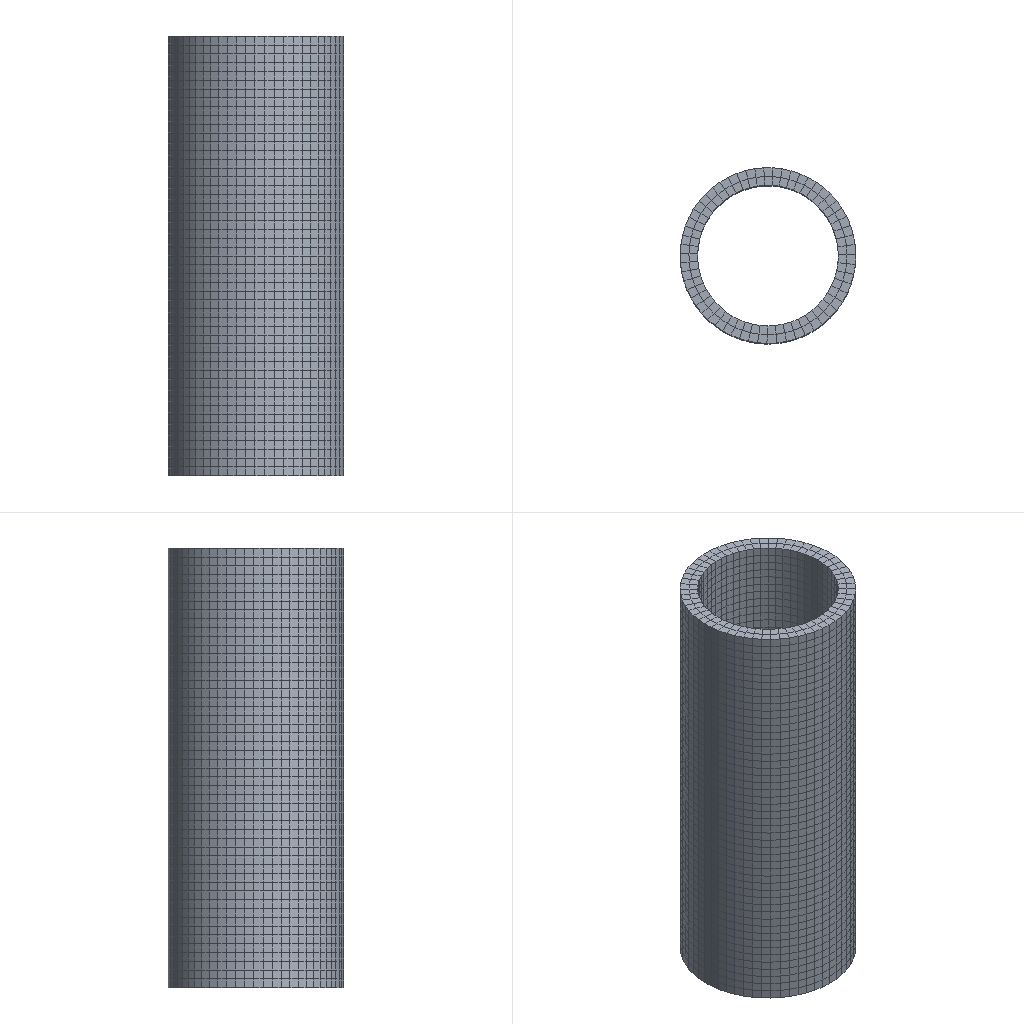Simulation study | abaqus
Set-up summary:
category,name,step,type,value,unit,region
solver,abaqus
solver,version,,,Abaqus/Standard 2020
units,not stated in the deck,,not stated
analysis,deck,,static,static
load_step,Step-1,Step-1,static
load_step,requested,,,1
mesh,nodes,,,8874
mesh,elements,,,5800
element_type,C3D8R,,solid,5800
load,load commands in deck,,count,1
bc,support commands in deck,,count,1
material,MATERIAL-1,,in results
check,setup vs results,,match,"per instance, exact: element labels, types and connectivity; labels of the nodes the elements use; coordinates of those nodes at SINGLE_PRECISION in 1 of 1 instance(s)"
Abaqus input file, long lists of numbers shortened:
*Heading
** Job name: Job-1 Model name: Model-1
** Generated by: Abaqus/CAE 2020
*Preprint, echo=NO, model=NO, history=NO, contact=NO
**
** PARTS
**
*Part, name=Part-1
*Node
      1,   14.315,   7.147,           0.
      2,   17.901,   8.919,           0.
** (8872 more lines like these left out)
*Element, type=C3D8R
   1,  175,  184,  295,  218,    1,   10,  121,   44
   2,  184,  176,  185,  295,   10,    2,   11,  121
** (5798 more lines like these left out)
*Nset, nset=Set-1, generate
    1,  8874,     1
*Elset, elset=Set-1, generate
    1,  5800,     1
** Section: Section-1
*Solid Section, elset=Set-1, material=Material-1
,
*End Part
**
**
** ASSEMBLY
**
*Assembly, name=Assembly
**
*Instance, name=Part-1-1, part=Part-1
*End Instance
**
*Nset, nset=Set-1, instance=Part-1-1
    1,    2,    3,    4,    5,    6,    7,    8,    9,   10,   11,   12,   13,   14,   15,   16
   17,   18,   19,   20,   21,   22,   23,   24,   25,   26,   27,   28,   29,   30,   31,   32
** (20 more lines like these left out)
*Elset, elset=Set-1, instance=Part-1-1
    1,    2,    3,    4,    5,    6,    7,    8,    9,   10,   11,   12,   13,   14,   15,   16
   17,   18,   19,   20,   21,   22,   23,   24,   25,   26,   27,   28,   29,   30,   31,   32
** (13 more lines like these left out)
*Elset, elset=_Surf-1_S6, internal, instance=Part-1-1
    1,    3,    5,    7,    9,   11,   13,   15,   17,   19,   21,   23,   25,   27,   29,   31
   33,   35,   37,   39,   41,   43,   45,   47,   49,   51,   53,   55,   57,   59,   61,   63
** (98 more lines like these left out)
*Elset, elset=_Surf-1_S4, internal, instance=Part-1-1
   66,   68,   70,   72,   74,   76,   78,   80,   82,   84,   86,   88,   90,   92,   94,   96
   98,  100,  102,  104,  106,  108,  110,  112,  114,  116,  182,  184,  186,  188,  190,  192
** (80 more lines like these left out)
*Surface, type=ELEMENT, name=Surf-1
_Surf-1_S6, S6
_Surf-1_S4, S4
*End Assembly
**
** MATERIALS
**
*Material, name=Material-1
*Elastic
 0.5, 0.49
** ----------------------------------------------------------------
**
** STEP: Step-1
**
*Step, name=Step-1, nlgeom=YES, inc=1000
*Static, stabilize=0.0002, allsdtol=0.05, continue=NO
0.01, 1., 1e-05, 1.
**
** BOUNDARY CONDITIONS
**
** Name: BC-1 Type: 位移/转角
*Boundary
Set-1, 3, 3
**
** LOADS
**
** Name: Load-1   Type: Pressure
*Dsload
Surf-1, P, 0.01
**
** OUTPUT REQUESTS
**
*Restart, write, frequency=0
**
** FIELD OUTPUT: F-Output-1
**
*Output, field
*Node Output
CF, RF, RM, RT, U, V
*Element Output, directions=YES
E, LE, MISES, MISESMAX, MISESONLY, PE, PEEQ, PEEQMAX, PEEQT, PEMAG, S, SSAVG
*Contact Output
CDISP, CSTRESS
**
** HISTORY OUTPUT: H-Output-1
**
*Output, history, variable=PRESELECT
*End Step
Results summary:
result,step,,completed,increments=11 time=1.0/1.0
result,analysis,,,static
result,last_loadstep,,,1
result,primary field,,,U
result,reaction total,,FX,0.0,model units
result,reaction total,,FY,0.0,model units
result,reaction total,,FZ,0.0,model units